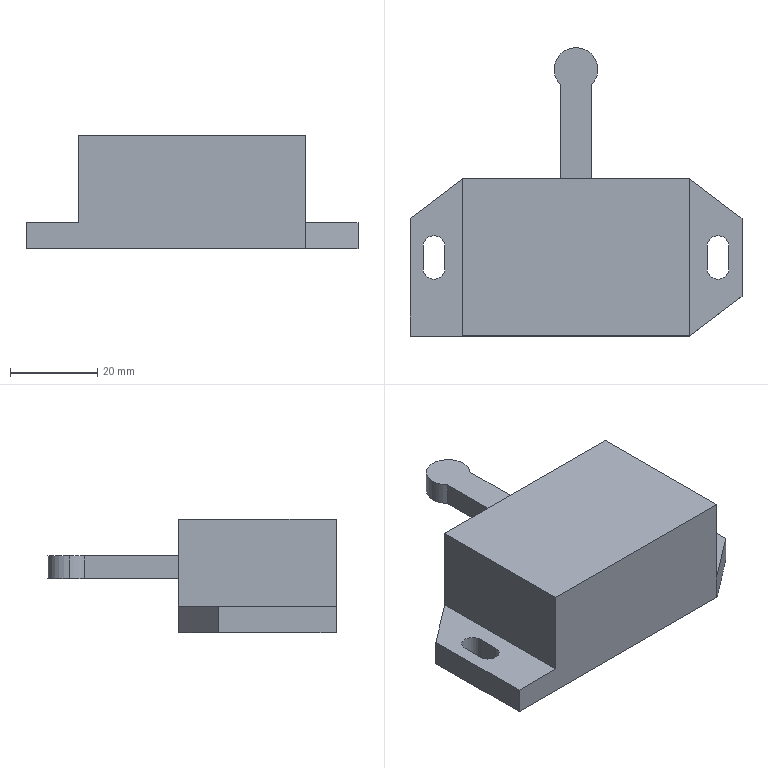Part | SolidWorks | features BaseBody 1 | 1 solid | 28 faces | box 76 x 66 x 26 mm | volume 53615 mm3 | plane 21 | cylinder 7 | commonest cylinder face diameters 5 x4 10 x3
STEP:
#1=CARTESIAN_POINT('',(-5.,43.,12.393));
#2=VERTEX_POINT('',#1);
#3=CARTESIAN_POINT('',(-5.,43.,17.607));
#4=VERTEX_POINT('',#3);
#5=CARTESIAN_POINT('',(-5.,43.,-1.75));
#6=DIRECTION('',(0.,0.,1.));
#7=VECTOR('',#6,1000.);
#8=LINE('',#5,#7);
#9=EDGE_CURVE('',#2,#4,#8,.T.);
#10=ORIENTED_EDGE('',*,*,#9,.F.);
#11=CARTESIAN_POINT('',(-3.61,39.541,12.393));
#12=VERTEX_POINT('',#11);
#13=CARTESIAN_POINT('',(0.,43.,12.393));
#14=DIRECTION('',(0.,0.,-1.));
#15=DIRECTION('',(1.,0.,0.));
#16=AXIS2_PLACEMENT_3D('',#13,#14,#15);
#17=CIRCLE('',#16,5.);
#18=EDGE_CURVE('',#12,#2,#17,.T.);
#19=ORIENTED_EDGE('',*,*,#18,.F.);
#20=CARTESIAN_POINT('',(-3.61,39.541,17.607));
#21=VERTEX_POINT('',#20);
#22=CARTESIAN_POINT('',(-3.61,39.541,-1.75));
#23=DIRECTION('',(0.,0.,-1.));
#24=VECTOR('',#23,1000.);
#25=LINE('',#22,#24);
#26=EDGE_CURVE('',#21,#12,#25,.T.);
#27=ORIENTED_EDGE('',*,*,#26,.F.);
#28=CARTESIAN_POINT('',(0.,43.,17.607));
#29=DIRECTION('',(0.,0.,1.));
#30=DIRECTION('',(1.,0.,0.));
#31=AXIS2_PLACEMENT_3D('',#28,#29,#30);
#32=CIRCLE('',#31,5.);
#33=EDGE_CURVE('',#4,#21,#32,.T.);
#34=ORIENTED_EDGE('',*,*,#33,.F.);
#35=EDGE_LOOP('',(#10,#19,#27,#34));
#36=FACE_OUTER_BOUND('',#35,.T.);
#37=CARTESIAN_POINT('',(0.,43.,-1.75));
#38=DIRECTION('',(0.,0.,1.));
#39=DIRECTION('',(1.,0.,0.));
#40=AXIS2_PLACEMENT_3D('',#37,#38,#39);
#41=CYLINDRICAL_SURFACE('',#40,5.);
#42=ADVANCED_FACE('',(#36),#41,.T.);
#43=CARTESIAN_POINT('',(3.61,39.541,17.607));
#44=VERTEX_POINT('',#43);
#45=CARTESIAN_POINT('',(3.61,18.,17.607));
#46=VERTEX_POINT('',#45);
#47=CARTESIAN_POINT('',(3.61,43.,17.607));
#48=DIRECTION('',(0.,-1.,0.));
#49=VECTOR('',#48,1000.);
#50=LINE('',#47,#49);
#51=EDGE_CURVE('',#44,#46,#50,.T.);
#52=ORIENTED_EDGE('',*,*,#51,.F.);
#53=CARTESIAN_POINT('',(5.,43.,17.607));
#54=VERTEX_POINT('',#53);
#55=CARTESIAN_POINT('',(0.,43.,17.607));
#56=DIRECTION('',(0.,0.,1.));
#57=DIRECTION('',(1.,0.,0.));
#58=AXIS2_PLACEMENT_3D('',#55,#56,#57);
#59=CIRCLE('',#58,5.);
#60=EDGE_CURVE('',#44,#54,#59,.T.);
#61=ORIENTED_EDGE('',*,*,#60,.T.);
#62=CARTESIAN_POINT('',(0.,43.,17.607));
#63=DIRECTION('',(0.,0.,1.));
#64=DIRECTION('',(1.,0.,0.));
#65=AXIS2_PLACEMENT_3D('',#62,#63,#64);
#66=CIRCLE('',#65,5.);
#67=EDGE_CURVE('',#54,#4,#66,.T.);
#68=ORIENTED_EDGE('',*,*,#67,.T.);
#69=ORIENTED_EDGE('',*,*,#33,.T.);
#70=CARTESIAN_POINT('',(-3.61,18.,17.607));
#71=VERTEX_POINT('',#70);
#72=CARTESIAN_POINT('',(-3.61,43.,17.607));
#73=DIRECTION('',(0.,-1.,0.));
#74=VECTOR('',#73,1000.);
#75=LINE('',#72,#74);
#76=EDGE_CURVE('',#21,#71,#75,.T.);
#77=ORIENTED_EDGE('',*,*,#76,.T.);
#78=CARTESIAN_POINT('',(-3.61,18.,17.607));
#79=DIRECTION('',(1.,0.,0.));
#80=VECTOR('',#79,1000.);
#81=LINE('',#78,#80);
#82=EDGE_CURVE('',#71,#46,#81,.T.);
#83=ORIENTED_EDGE('',*,*,#82,.T.);
#84=EDGE_LOOP('',(#52,#61,#68,#69,#77,#83));
#85=FACE_OUTER_BOUND('',#84,.T.);
#86=CARTESIAN_POINT('',(-3.61,43.,17.607));
#87=DIRECTION('',(0.,0.,-1.));
#88=DIRECTION('',(-1.,0.,0.));
#89=AXIS2_PLACEMENT_3D('',#86,#87,#88);
#90=PLANE('',#89);
#91=ADVANCED_FACE('',(#85),#90,.F.);
#92=ORIENTED_EDGE('',*,*,#76,.F.);
#93=ORIENTED_EDGE('',*,*,#26,.T.);
#94=CARTESIAN_POINT('',(-3.61,18.,12.393));
#95=VERTEX_POINT('',#94);
#96=CARTESIAN_POINT('',(-3.61,43.,12.393));
#97=DIRECTION('',(0.,-1.,0.));
#98=VECTOR('',#97,1000.);
#99=LINE('',#96,#98);
#100=EDGE_CURVE('',#12,#95,#99,.T.);
#101=ORIENTED_EDGE('',*,*,#100,.T.);
#102=CARTESIAN_POINT('',(-3.61,18.,12.393));
#103=DIRECTION('',(0.,0.,1.));
#104=VECTOR('',#103,1000.);
#105=LINE('',#102,#104);
#106=EDGE_CURVE('',#95,#71,#105,.T.);
#107=ORIENTED_EDGE('',*,*,#106,.T.);
#108=EDGE_LOOP('',(#92,#93,#101,#107));
#109=FACE_OUTER_BOUND('',#108,.T.);
#110=CARTESIAN_POINT('',(-3.61,43.,12.393));
#111=DIRECTION('',(1.,0.,0.));
#112=DIRECTION('',(0.,1.,0.));
#113=AXIS2_PLACEMENT_3D('',#110,#111,#112);
#114=PLANE('',#113);
#115=ADVANCED_FACE('',(#109),#114,.F.);
#116=ORIENTED_EDGE('',*,*,#18,.T.);
#117=CARTESIAN_POINT('',(5.,43.,12.393));
#118=VERTEX_POINT('',#117);
#119=CARTESIAN_POINT('',(0.,43.,12.393));
#120=DIRECTION('',(0.,0.,-1.));
#121=DIRECTION('',(1.,0.,0.));
#122=AXIS2_PLACEMENT_3D('',#119,#120,#121);
#123=CIRCLE('',#122,5.);
#124=EDGE_CURVE('',#2,#118,#123,.T.);
#125=ORIENTED_EDGE('',*,*,#124,.T.);
#126=CARTESIAN_POINT('',(3.61,39.541,12.393));
#127=VERTEX_POINT('',#126);
#128=CARTESIAN_POINT('',(0.,43.,12.393));
#129=DIRECTION('',(0.,0.,-1.));
#130=DIRECTION('',(1.,0.,0.));
#131=AXIS2_PLACEMENT_3D('',#128,#129,#130);
#132=CIRCLE('',#131,5.);
#133=EDGE_CURVE('',#118,#127,#132,.T.);
#134=ORIENTED_EDGE('',*,*,#133,.T.);
#135=CARTESIAN_POINT('',(3.61,18.,12.393));
#136=VERTEX_POINT('',#135);
#137=CARTESIAN_POINT('',(3.61,43.,12.393));
#138=DIRECTION('',(0.,-1.,0.));
#139=VECTOR('',#138,1000.);
#140=LINE('',#137,#139);
#141=EDGE_CURVE('',#127,#136,#140,.T.);
#142=ORIENTED_EDGE('',*,*,#141,.T.);
#143=CARTESIAN_POINT('',(-3.61,18.,12.393));
#144=DIRECTION('',(-1.,0.,0.));
#145=VECTOR('',#144,1000.);
#146=LINE('',#143,#145);
#147=EDGE_CURVE('',#136,#95,#146,.T.);
#148=ORIENTED_EDGE('',*,*,#147,.T.);
#149=ORIENTED_EDGE('',*,*,#100,.F.);
#150=EDGE_LOOP('',(#116,#125,#134,#142,#148,#149));
#151=FACE_OUTER_BOUND('',#150,.T.);
#152=CARTESIAN_POINT('',(-3.61,43.,12.393));
#153=DIRECTION('',(0.,0.,1.));
#154=DIRECTION('',(1.,0.,0.));
#155=AXIS2_PLACEMENT_3D('',#152,#153,#154);
#156=PLANE('',#155);
#157=ADVANCED_FACE('',(#151),#156,.F.);
#158=ORIENTED_EDGE('',*,*,#141,.F.);
#159=CARTESIAN_POINT('',(3.61,39.541,-1.75));
#160=DIRECTION('',(0.,0.,1.));
#161=VECTOR('',#160,1000.);
#162=LINE('',#159,#161);
#163=EDGE_CURVE('',#127,#44,#162,.T.);
#164=ORIENTED_EDGE('',*,*,#163,.T.);
#165=ORIENTED_EDGE('',*,*,#51,.T.);
#166=CARTESIAN_POINT('',(3.61,18.,12.393));
#167=DIRECTION('',(0.,0.,-1.));
#168=VECTOR('',#167,1000.);
#169=LINE('',#166,#168);
#170=EDGE_CURVE('',#46,#136,#169,.T.);
#171=ORIENTED_EDGE('',*,*,#170,.T.);
#172=EDGE_LOOP('',(#158,#164,#165,#171));
#173=FACE_OUTER_BOUND('',#172,.T.);
#174=CARTESIAN_POINT('',(3.61,43.,12.393));
#175=DIRECTION('',(-1.,0.,0.));
#176=DIRECTION('',(0.,1.,0.));
#177=AXIS2_PLACEMENT_3D('',#174,#175,#176);
#178=PLANE('',#177);
#179=ADVANCED_FACE('',(#173),#178,.F.);
#180=CARTESIAN_POINT('',(26.062,-18.,26.));
#181=VERTEX_POINT('',#180);
#182=CARTESIAN_POINT('',(26.062,18.,26.));
#183=VERTEX_POINT('',#182);
#184=CARTESIAN_POINT('',(26.062,-18.,26.));
#185=DIRECTION('',(0.,1.,0.));
#186=VECTOR('',#185,1000.);
#187=LINE('',#184,#186);
#188=EDGE_CURVE('',#181,#183,#187,.T.);
#189=ORIENTED_EDGE('',*,*,#188,.T.);
#190=CARTESIAN_POINT('',(-26.062,18.,26.));
#191=VERTEX_POINT('',#190);
#192=CARTESIAN_POINT('',(-26.062,18.,26.));
#193=DIRECTION('',(-1.,0.,0.));
#194=VECTOR('',#193,1000.);
#195=LINE('',#192,#194);
#196=EDGE_CURVE('',#183,#191,#195,.T.);
#197=ORIENTED_EDGE('',*,*,#196,.T.);
#198=CARTESIAN_POINT('',(-26.062,-18.,26.));
#199=VERTEX_POINT('',#198);
#200=CARTESIAN_POINT('',(-26.062,-18.,26.));
#201=DIRECTION('',(0.,-1.,0.));
#202=VECTOR('',#201,1000.);
#203=LINE('',#200,#202);
#204=EDGE_CURVE('',#191,#199,#203,.T.);
#205=ORIENTED_EDGE('',*,*,#204,.T.);
#206=CARTESIAN_POINT('',(-26.062,-18.,26.));
#207=DIRECTION('',(1.,0.,0.));
#208=VECTOR('',#207,1000.);
#209=LINE('',#206,#208);
#210=EDGE_CURVE('',#199,#181,#209,.T.);
#211=ORIENTED_EDGE('',*,*,#210,.T.);
#212=EDGE_LOOP('',(#189,#197,#205,#211));
#213=FACE_OUTER_BOUND('',#212,.T.);
#214=CARTESIAN_POINT('',(0.,0.,26.));
#215=DIRECTION('',(0.,0.,-1.));
#216=DIRECTION('',(0.,-1.,0.));
#217=AXIS2_PLACEMENT_3D('',#214,#215,#216);
#218=PLANE('',#217);
#219=ADVANCED_FACE('',(#213),#218,.F.);
#220=CARTESIAN_POINT('',(-26.062,18.,6.));
#221=VERTEX_POINT('',#220);
#222=CARTESIAN_POINT('',(-26.062,-18.,6.));
#223=VERTEX_POINT('',#222);
#224=CARTESIAN_POINT('',(-26.062,-18.,6.));
#225=DIRECTION('',(0.,-1.,0.));
#226=VECTOR('',#225,1000.);
#227=LINE('',#224,#226);
#228=EDGE_CURVE('',#221,#223,#227,.T.);
#229=ORIENTED_EDGE('',*,*,#228,.T.);
#230=CARTESIAN_POINT('',(-26.062,-18.,26.));
#231=DIRECTION('',(0.,0.,-1.));
#232=VECTOR('',#231,1000.);
#233=LINE('',#230,#232);
#234=EDGE_CURVE('',#199,#223,#233,.T.);
#235=ORIENTED_EDGE('',*,*,#234,.F.);
#236=ORIENTED_EDGE('',*,*,#204,.F.);
#237=CARTESIAN_POINT('',(-26.062,18.,26.));
#238=DIRECTION('',(0.,0.,-1.));
#239=VECTOR('',#238,1000.);
#240=LINE('',#237,#239);
#241=EDGE_CURVE('',#191,#221,#240,.T.);
#242=ORIENTED_EDGE('',*,*,#241,.T.);
#243=EDGE_LOOP('',(#229,#235,#236,#242));
#244=FACE_OUTER_BOUND('',#243,.T.);
#245=CARTESIAN_POINT('',(-26.062,-18.,26.));
#246=DIRECTION('',(1.,0.,0.));
#247=DIRECTION('',(0.,1.,0.));
#248=AXIS2_PLACEMENT_3D('',#245,#246,#247);
#249=PLANE('',#248);
#250=ADVANCED_FACE('',(#244),#249,.F.);
#251=CARTESIAN_POINT('',(26.062,-18.,6.));
#252=VERTEX_POINT('',#251);
#253=CARTESIAN_POINT('',(26.062,18.,6.));
#254=VERTEX_POINT('',#253);
#255=CARTESIAN_POINT('',(26.062,-18.,6.));
#256=DIRECTION('',(0.,1.,0.));
#257=VECTOR('',#256,1000.);
#258=LINE('',#255,#257);
#259=EDGE_CURVE('',#252,#254,#258,.T.);
#260=ORIENTED_EDGE('',*,*,#259,.T.);
#261=CARTESIAN_POINT('',(26.062,18.,26.));
#262=DIRECTION('',(0.,0.,-1.));
#263=VECTOR('',#262,1000.);
#264=LINE('',#261,#263);
#265=EDGE_CURVE('',#183,#254,#264,.T.);
#266=ORIENTED_EDGE('',*,*,#265,.F.);
#267=ORIENTED_EDGE('',*,*,#188,.F.);
#268=CARTESIAN_POINT('',(26.062,-18.,26.));
#269=DIRECTION('',(0.,0.,-1.));
#270=VECTOR('',#269,1000.);
#271=LINE('',#268,#270);
#272=EDGE_CURVE('',#181,#252,#271,.T.);
#273=ORIENTED_EDGE('',*,*,#272,.T.);
#274=EDGE_LOOP('',(#260,#266,#267,#273));
#275=FACE_OUTER_BOUND('',#274,.T.);
#276=CARTESIAN_POINT('',(26.062,-18.,26.));
#277=DIRECTION('',(-1.,0.,0.));
#278=DIRECTION('',(0.,0.,1.));
#279=AXIS2_PLACEMENT_3D('',#276,#277,#278);
#280=PLANE('',#279);
#281=ADVANCED_FACE('',(#275),#280,.F.);
#282=CARTESIAN_POINT('',(35.,-2.5,0.));
#283=VERTEX_POINT('',#282);
#284=CARTESIAN_POINT('',(35.,2.5,0.));
#285=VERTEX_POINT('',#284);
#286=CARTESIAN_POINT('',(35.,2.5,0.));
#287=DIRECTION('',(0.,1.,0.));
#288=VECTOR('',#287,1000.);
#289=LINE('',#286,#288);
#290=EDGE_CURVE('',#283,#285,#289,.T.);
#291=ORIENTED_EDGE('',*,*,#290,.F.);
#292=CARTESIAN_POINT('',(35.,-2.5,6.));
#293=VERTEX_POINT('',#292);
#294=CARTESIAN_POINT('',(35.,-2.5,6.));
#295=DIRECTION('',(0.,0.,-1.));
#296=VECTOR('',#295,1000.);
#297=LINE('',#294,#296);
#298=EDGE_CURVE('',#293,#283,#297,.T.);
#299=ORIENTED_EDGE('',*,*,#298,.F.);
#300=CARTESIAN_POINT('',(35.,2.5,6.));
#301=VERTEX_POINT('',#300);
#302=CARTESIAN_POINT('',(35.,2.5,6.));
#303=DIRECTION('',(0.,1.,0.));
#304=VECTOR('',#303,1000.);
#305=LINE('',#302,#304);
#306=EDGE_CURVE('',#293,#301,#305,.T.);
#307=ORIENTED_EDGE('',*,*,#306,.T.);
#308=CARTESIAN_POINT('',(35.,2.5,6.));
#309=DIRECTION('',(0.,0.,-1.));
#310=VECTOR('',#309,1000.);
#311=LINE('',#308,#310);
#312=EDGE_CURVE('',#301,#285,#311,.T.);
#313=ORIENTED_EDGE('',*,*,#312,.T.);
#314=EDGE_LOOP('',(#291,#299,#307,#313));
#315=FACE_OUTER_BOUND('',#314,.T.);
#316=CARTESIAN_POINT('',(35.,2.5,6.));
#317=DIRECTION('',(-1.,0.,0.));
#318=DIRECTION('',(0.,0.,1.));
#319=AXIS2_PLACEMENT_3D('',#316,#317,#318);
#320=PLANE('',#319);
#321=ADVANCED_FACE('',(#315),#320,.T.);
#322=CARTESIAN_POINT('',(30.,-2.5,0.));
#323=VERTEX_POINT('',#322);
#324=CARTESIAN_POINT('',(32.5,-2.5,0.));
#325=DIRECTION('',(0.,0.,1.));
#326=DIRECTION('',(-1.,0.,0.));
#327=AXIS2_PLACEMENT_3D('',#324,#325,#326);
#328=CIRCLE('',#327,2.5);
#329=EDGE_CURVE('',#323,#283,#328,.T.);
#330=ORIENTED_EDGE('',*,*,#329,.F.);
#331=CARTESIAN_POINT('',(30.,-2.5,6.));
#332=VERTEX_POINT('',#331);
#333=CARTESIAN_POINT('',(30.,-2.5,6.));
#334=DIRECTION('',(0.,0.,-1.));
#335=VECTOR('',#334,1000.);
#336=LINE('',#333,#335);
#337=EDGE_CURVE('',#332,#323,#336,.T.);
#338=ORIENTED_EDGE('',*,*,#337,.F.);
#339=CARTESIAN_POINT('',(32.5,-2.5,6.));
#340=DIRECTION('',(0.,0.,1.));
#341=DIRECTION('',(-1.,0.,0.));
#342=AXIS2_PLACEMENT_3D('',#339,#340,#341);
#343=CIRCLE('',#342,2.5);
#344=EDGE_CURVE('',#332,#293,#343,.T.);
#345=ORIENTED_EDGE('',*,*,#344,.T.);
#346=ORIENTED_EDGE('',*,*,#298,.T.);
#347=EDGE_LOOP('',(#330,#338,#345,#346));
#348=FACE_OUTER_BOUND('',#347,.T.);
#349=CARTESIAN_POINT('',(32.5,-2.5,6.));
#350=DIRECTION('',(0.,0.,-1.));
#351=DIRECTION('',(-1.,0.,0.));
#352=AXIS2_PLACEMENT_3D('',#349,#350,#351);
#353=CYLINDRICAL_SURFACE('',#352,2.5);
#354=ADVANCED_FACE('',(#348),#353,.F.);
#355=CARTESIAN_POINT('',(30.,2.5,0.));
#356=VERTEX_POINT('',#355);
#357=CARTESIAN_POINT('',(30.,2.5,0.));
#358=DIRECTION('',(0.,-1.,0.));
#359=VECTOR('',#358,1000.);
#360=LINE('',#357,#359);
#361=EDGE_CURVE('',#356,#323,#360,.T.);
#362=ORIENTED_EDGE('',*,*,#361,.F.);
#363=CARTESIAN_POINT('',(30.,2.5,6.));
#364=VERTEX_POINT('',#363);
#365=CARTESIAN_POINT('',(30.,2.5,6.));
#366=DIRECTION('',(0.,0.,-1.));
#367=VECTOR('',#366,1000.);
#368=LINE('',#365,#367);
#369=EDGE_CURVE('',#364,#356,#368,.T.);
#370=ORIENTED_EDGE('',*,*,#369,.F.);
#371=CARTESIAN_POINT('',(30.,2.5,6.));
#372=DIRECTION('',(0.,-1.,0.));
#373=VECTOR('',#372,1000.);
#374=LINE('',#371,#373);
#375=EDGE_CURVE('',#364,#332,#374,.T.);
#376=ORIENTED_EDGE('',*,*,#375,.T.);
#377=ORIENTED_EDGE('',*,*,#337,.T.);
#378=EDGE_LOOP('',(#362,#370,#376,#377));
#379=FACE_OUTER_BOUND('',#378,.T.);
#380=CARTESIAN_POINT('',(30.,2.5,6.));
#381=DIRECTION('',(1.,0.,0.));
#382=DIRECTION('',(0.,1.,0.));
#383=AXIS2_PLACEMENT_3D('',#380,#381,#382);
#384=PLANE('',#383);
#385=ADVANCED_FACE('',(#379),#384,.T.);
#386=CARTESIAN_POINT('',(32.5,2.5,0.));
#387=DIRECTION('',(0.,0.,1.));
#388=DIRECTION('',(-1.,0.,0.));
#389=AXIS2_PLACEMENT_3D('',#386,#387,#388);
#390=CIRCLE('',#389,2.5);
#391=EDGE_CURVE('',#285,#356,#390,.T.);
#392=ORIENTED_EDGE('',*,*,#391,.F.);
#393=ORIENTED_EDGE('',*,*,#312,.F.);
#394=CARTESIAN_POINT('',(32.5,2.5,6.));
#395=DIRECTION('',(0.,0.,1.));
#396=DIRECTION('',(-1.,0.,0.));
#397=AXIS2_PLACEMENT_3D('',#394,#395,#396);
#398=CIRCLE('',#397,2.5);
#399=EDGE_CURVE('',#301,#364,#398,.T.);
#400=ORIENTED_EDGE('',*,*,#399,.T.);
#401=ORIENTED_EDGE('',*,*,#369,.T.);
#402=EDGE_LOOP('',(#392,#393,#400,#401));
#403=FACE_OUTER_BOUND('',#402,.T.);
#404=CARTESIAN_POINT('',(32.5,2.5,6.));
#405=DIRECTION('',(0.,0.,-1.));
#406=DIRECTION('',(-1.,0.,0.));
#407=AXIS2_PLACEMENT_3D('',#404,#405,#406);
#408=CYLINDRICAL_SURFACE('',#407,2.5);
#409=ADVANCED_FACE('',(#403),#408,.F.);
#410=CARTESIAN_POINT('',(-30.,-2.5,0.));
#411=VERTEX_POINT('',#410);
#412=CARTESIAN_POINT('',(-30.,2.5,0.));
#413=VERTEX_POINT('',#412);
#414=CARTESIAN_POINT('',(-30.,2.5,0.));
#415=DIRECTION('',(0.,1.,0.));
#416=VECTOR('',#415,1000.);
#417=LINE('',#414,#416);
#418=EDGE_CURVE('',#411,#413,#417,.T.);
#419=ORIENTED_EDGE('',*,*,#418,.F.);
#420=CARTESIAN_POINT('',(-30.,-2.5,6.));
#421=VERTEX_POINT('',#420);
#422=CARTESIAN_POINT('',(-30.,-2.5,6.));
#423=DIRECTION('',(0.,0.,-1.));
#424=VECTOR('',#423,1000.);
#425=LINE('',#422,#424);
#426=EDGE_CURVE('',#421,#411,#425,.T.);
#427=ORIENTED_EDGE('',*,*,#426,.F.);
#428=CARTESIAN_POINT('',(-30.,2.5,6.));
#429=VERTEX_POINT('',#428);
#430=CARTESIAN_POINT('',(-30.,2.5,6.));
#431=DIRECTION('',(0.,1.,0.));
#432=VECTOR('',#431,1000.);
#433=LINE('',#430,#432);
#434=EDGE_CURVE('',#421,#429,#433,.T.);
#435=ORIENTED_EDGE('',*,*,#434,.T.);
#436=CARTESIAN_POINT('',(-30.,2.5,6.));
#437=DIRECTION('',(0.,0.,-1.));
#438=VECTOR('',#437,1000.);
#439=LINE('',#436,#438);
#440=EDGE_CURVE('',#429,#413,#439,.T.);
#441=ORIENTED_EDGE('',*,*,#440,.T.);
#442=EDGE_LOOP('',(#419,#427,#435,#441));
#443=FACE_OUTER_BOUND('',#442,.T.);
#444=CARTESIAN_POINT('',(-30.,2.5,6.));
#445=DIRECTION('',(-1.,0.,0.));
#446=DIRECTION('',(0.,0.,1.));
#447=AXIS2_PLACEMENT_3D('',#444,#445,#446);
#448=PLANE('',#447);
#449=ADVANCED_FACE('',(#443),#448,.T.);
#450=CARTESIAN_POINT('',(-35.,-2.5,0.));
#451=VERTEX_POINT('',#450);
#452=CARTESIAN_POINT('',(-32.5,-2.5,0.));
#453=DIRECTION('',(0.,0.,1.));
#454=DIRECTION('',(1.,0.,0.));
#455=AXIS2_PLACEMENT_3D('',#452,#453,#454);
#456=CIRCLE('',#455,2.5);
#457=EDGE_CURVE('',#451,#411,#456,.T.);
#458=ORIENTED_EDGE('',*,*,#457,.F.);
#459=CARTESIAN_POINT('',(-35.,-2.5,6.));
#460=VERTEX_POINT('',#459);
#461=CARTESIAN_POINT('',(-35.,-2.5,6.));
#462=DIRECTION('',(0.,0.,-1.));
#463=VECTOR('',#462,1000.);
#464=LINE('',#461,#463);
#465=EDGE_CURVE('',#460,#451,#464,.T.);
#466=ORIENTED_EDGE('',*,*,#465,.F.);
#467=CARTESIAN_POINT('',(-32.5,-2.5,6.));
#468=DIRECTION('',(0.,0.,1.));
#469=DIRECTION('',(1.,0.,0.));
#470=AXIS2_PLACEMENT_3D('',#467,#468,#469);
#471=CIRCLE('',#470,2.5);
#472=EDGE_CURVE('',#460,#421,#471,.T.);
#473=ORIENTED_EDGE('',*,*,#472,.T.);
#474=ORIENTED_EDGE('',*,*,#426,.T.);
#475=EDGE_LOOP('',(#458,#466,#473,#474));
#476=FACE_OUTER_BOUND('',#475,.T.);
#477=CARTESIAN_POINT('',(-32.5,-2.5,6.));
#478=DIRECTION('',(0.,0.,-1.));
#479=DIRECTION('',(-1.,0.,0.));
#480=AXIS2_PLACEMENT_3D('',#477,#478,#479);
#481=CYLINDRICAL_SURFACE('',#480,2.5);
#482=ADVANCED_FACE('',(#476),#481,.F.);
#483=CARTESIAN_POINT('',(-35.,2.5,0.));
#484=VERTEX_POINT('',#483);
#485=CARTESIAN_POINT('',(-35.,2.5,0.));
#486=DIRECTION('',(0.,-1.,0.));
#487=VECTOR('',#486,1000.);
#488=LINE('',#485,#487);
#489=EDGE_CURVE('',#484,#451,#488,.T.);
#490=ORIENTED_EDGE('',*,*,#489,.F.);
#491=CARTESIAN_POINT('',(-35.,2.5,6.));
#492=VERTEX_POINT('',#491);
#493=CARTESIAN_POINT('',(-35.,2.5,6.));
#494=DIRECTION('',(0.,0.,-1.));
#495=VECTOR('',#494,1000.);
#496=LINE('',#493,#495);
#497=EDGE_CURVE('',#492,#484,#496,.T.);
#498=ORIENTED_EDGE('',*,*,#497,.F.);
#499=CARTESIAN_POINT('',(-35.,2.5,6.));
#500=DIRECTION('',(0.,-1.,0.));
#501=VECTOR('',#500,1000.);
#502=LINE('',#499,#501);
#503=EDGE_CURVE('',#492,#460,#502,.T.);
#504=ORIENTED_EDGE('',*,*,#503,.T.);
#505=ORIENTED_EDGE('',*,*,#465,.T.);
#506=EDGE_LOOP('',(#490,#498,#504,#505));
#507=FACE_OUTER_BOUND('',#506,.T.);
#508=CARTESIAN_POINT('',(-35.,2.5,6.));
#509=DIRECTION('',(1.,0.,0.));
#510=DIRECTION('',(0.,1.,0.));
#511=AXIS2_PLACEMENT_3D('',#508,#509,#510);
#512=PLANE('',#511);
#513=ADVANCED_FACE('',(#507),#512,.T.);
#514=CARTESIAN_POINT('',(-32.5,2.5,0.));
#515=DIRECTION('',(0.,0.,1.));
#516=DIRECTION('',(1.,0.,0.));
#517=AXIS2_PLACEMENT_3D('',#514,#515,#516);
#518=CIRCLE('',#517,2.5);
#519=EDGE_CURVE('',#413,#484,#518,.T.);
#520=ORIENTED_EDGE('',*,*,#519,.F.);
#521=ORIENTED_EDGE('',*,*,#440,.F.);
#522=CARTESIAN_POINT('',(-32.5,2.5,6.));
#523=DIRECTION('',(0.,0.,1.));
#524=DIRECTION('',(1.,0.,0.));
#525=AXIS2_PLACEMENT_3D('',#522,#523,#524);
#526=CIRCLE('',#525,2.5);
#527=EDGE_CURVE('',#429,#492,#526,.T.);
#528=ORIENTED_EDGE('',*,*,#527,.T.);
#529=ORIENTED_EDGE('',*,*,#497,.T.);
#530=EDGE_LOOP('',(#520,#521,#528,#529));
#531=FACE_OUTER_BOUND('',#530,.T.);
#532=CARTESIAN_POINT('',(-32.5,2.5,6.));
#533=DIRECTION('',(0.,0.,-1.));
#534=DIRECTION('',(-1.,0.,0.));
#535=AXIS2_PLACEMENT_3D('',#532,#533,#534);
#536=CYLINDRICAL_SURFACE('',#535,2.5);
#537=ADVANCED_FACE('',(#531),#536,.F.);
#538=CARTESIAN_POINT('',(-38.,8.923,0.));
#539=VERTEX_POINT('',#538);
#540=CARTESIAN_POINT('',(-38.,-18.,0.));
#541=VERTEX_POINT('',#540);
#542=CARTESIAN_POINT('',(-38.,8.923,0.));
#543=DIRECTION('',(0.,-1.,0.));
#544=VECTOR('',#543,1000.);
#545=LINE('',#542,#544);
#546=EDGE_CURVE('',#539,#541,#545,.T.);
#547=ORIENTED_EDGE('',*,*,#546,.T.);
#548=CARTESIAN_POINT('',(-38.,-18.,6.));
#549=VERTEX_POINT('',#548);
#550=CARTESIAN_POINT('',(-38.,-18.,6.));
#551=DIRECTION('',(0.,0.,-1.));
#552=VECTOR('',#551,1000.);
#553=LINE('',#550,#552);
#554=EDGE_CURVE('',#549,#541,#553,.T.);
#555=ORIENTED_EDGE('',*,*,#554,.F.);
#556=CARTESIAN_POINT('',(-38.,8.923,6.));
#557=VERTEX_POINT('',#556);
#558=CARTESIAN_POINT('',(-38.,8.923,6.));
#559=DIRECTION('',(0.,-1.,0.));
#560=VECTOR('',#559,1000.);
#561=LINE('',#558,#560);
#562=EDGE_CURVE('',#557,#549,#561,.T.);
#563=ORIENTED_EDGE('',*,*,#562,.F.);
#564=CARTESIAN_POINT('',(-38.,8.923,6.));
#565=DIRECTION('',(0.,0.,-1.));
#566=VECTOR('',#565,1000.);
#567=LINE('',#564,#566);
#568=EDGE_CURVE('',#557,#539,#567,.T.);
#569=ORIENTED_EDGE('',*,*,#568,.T.);
#570=EDGE_LOOP('',(#547,#555,#563,#569));
#571=FACE_OUTER_BOUND('',#570,.T.);
#572=CARTESIAN_POINT('',(-38.,8.923,6.));
#573=DIRECTION('',(1.,0.,0.));
#574=DIRECTION('',(0.,-1.,0.));
#575=AXIS2_PLACEMENT_3D('',#572,#573,#574);
#576=PLANE('',#575);
#577=ADVANCED_FACE('',(#571),#576,.F.);
#578=CARTESIAN_POINT('',(-26.062,18.,0.));
#579=VERTEX_POINT('',#578);
#580=CARTESIAN_POINT('',(-26.062,18.,0.));
#581=DIRECTION('',(-0.796,-0.6053,0.));
#582=VECTOR('',#581,1000.);
#583=LINE('',#580,#582);
#584=EDGE_CURVE('',#579,#539,#583,.T.);
#585=ORIENTED_EDGE('',*,*,#584,.T.);
#586=ORIENTED_EDGE('',*,*,#568,.F.);
#587=CARTESIAN_POINT('',(-26.062,18.,6.));
#588=DIRECTION('',(-0.796,-0.6053,0.));
#589=VECTOR('',#588,1000.);
#590=LINE('',#587,#589);
#591=EDGE_CURVE('',#221,#557,#590,.T.);
#592=ORIENTED_EDGE('',*,*,#591,.F.);
#593=CARTESIAN_POINT('',(-26.062,18.,6.));
#594=DIRECTION('',(0.,0.,-1.));
#595=VECTOR('',#594,1000.);
#596=LINE('',#593,#595);
#597=EDGE_CURVE('',#221,#579,#596,.T.);
#598=ORIENTED_EDGE('',*,*,#597,.T.);
#599=EDGE_LOOP('',(#585,#586,#592,#598));
#600=FACE_OUTER_BOUND('',#599,.T.);
#601=CARTESIAN_POINT('',(-26.062,18.,6.));
#602=DIRECTION('',(0.6053,-0.796,0.));
#603=DIRECTION('',(0.,0.,-1.));
#604=AXIS2_PLACEMENT_3D('',#601,#602,#603);
#605=PLANE('',#604);
#606=ADVANCED_FACE('',(#600),#605,.F.);
#607=CARTESIAN_POINT('',(38.,8.923,0.));
#608=VERTEX_POINT('',#607);
#609=CARTESIAN_POINT('',(26.062,18.,0.));
#610=VERTEX_POINT('',#609);
#611=CARTESIAN_POINT('',(26.062,18.,0.));
#612=DIRECTION('',(-0.796,0.6053,0.));
#613=VECTOR('',#612,1000.);
#614=LINE('',#611,#613);
#615=EDGE_CURVE('',#608,#610,#614,.T.);
#616=ORIENTED_EDGE('',*,*,#615,.T.);
#617=CARTESIAN_POINT('',(26.062,18.,6.));
#618=DIRECTION('',(0.,0.,-1.));
#619=VECTOR('',#618,1000.);
#620=LINE('',#617,#619);
#621=EDGE_CURVE('',#254,#610,#620,.T.);
#622=ORIENTED_EDGE('',*,*,#621,.F.);
#623=CARTESIAN_POINT('',(38.,8.923,6.));
#624=VERTEX_POINT('',#623);
#625=CARTESIAN_POINT('',(26.062,18.,6.));
#626=DIRECTION('',(-0.796,0.6053,0.));
#627=VECTOR('',#626,1000.);
#628=LINE('',#625,#627);
#629=EDGE_CURVE('',#624,#254,#628,.T.);
#630=ORIENTED_EDGE('',*,*,#629,.F.);
#631=CARTESIAN_POINT('',(38.,8.923,6.));
#632=DIRECTION('',(0.,0.,-1.));
#633=VECTOR('',#632,1000.);
#634=LINE('',#631,#633);
#635=EDGE_CURVE('',#624,#608,#634,.T.);
#636=ORIENTED_EDGE('',*,*,#635,.T.);
#637=EDGE_LOOP('',(#616,#622,#630,#636));
#638=FACE_OUTER_BOUND('',#637,.T.);
#639=CARTESIAN_POINT('',(26.062,18.,6.));
#640=DIRECTION('',(-0.6053,-0.796,0.));
#641=DIRECTION('',(-0.796,0.6053,0.));
#642=AXIS2_PLACEMENT_3D('',#639,#640,#641);
#643=PLANE('',#642);
#644=ADVANCED_FACE('',(#638),#643,.F.);
#645=CARTESIAN_POINT('',(38.,-8.923,0.));
#646=VERTEX_POINT('',#645);
#647=CARTESIAN_POINT('',(38.,8.923,0.));
#648=DIRECTION('',(0.,1.,0.));
#649=VECTOR('',#648,1000.);
#650=LINE('',#647,#649);
#651=EDGE_CURVE('',#646,#608,#650,.T.);
#652=ORIENTED_EDGE('',*,*,#651,.T.);
#653=ORIENTED_EDGE('',*,*,#635,.F.);
#654=CARTESIAN_POINT('',(38.,-8.923,6.));
#655=VERTEX_POINT('',#654);
#656=CARTESIAN_POINT('',(38.,8.923,6.));
#657=DIRECTION('',(0.,1.,0.));
#658=VECTOR('',#657,1000.);
#659=LINE('',#656,#658);
#660=EDGE_CURVE('',#655,#624,#659,.T.);
#661=ORIENTED_EDGE('',*,*,#660,.F.);
#662=CARTESIAN_POINT('',(38.,-8.923,6.));
#663=DIRECTION('',(0.,0.,-1.));
#664=VECTOR('',#663,1000.);
#665=LINE('',#662,#664);
#666=EDGE_CURVE('',#655,#646,#665,.T.);
#667=ORIENTED_EDGE('',*,*,#666,.T.);
#668=EDGE_LOOP('',(#652,#653,#661,#667));
#669=FACE_OUTER_BOUND('',#668,.T.);
#670=CARTESIAN_POINT('',(38.,8.923,6.));
#671=DIRECTION('',(-1.,0.,0.));
#672=DIRECTION('',(0.,0.,1.));
#673=AXIS2_PLACEMENT_3D('',#670,#671,#672);
#674=PLANE('',#673);
#675=ADVANCED_FACE('',(#669),#674,.F.);
#676=CARTESIAN_POINT('',(26.062,-18.,0.));
#677=VERTEX_POINT('',#676);
#678=CARTESIAN_POINT('',(26.062,-18.,0.));
#679=DIRECTION('',(0.796,0.6053,0.));
#680=VECTOR('',#679,1000.);
#681=LINE('',#678,#680);
#682=EDGE_CURVE('',#677,#646,#681,.T.);
#683=ORIENTED_EDGE('',*,*,#682,.T.);
#684=ORIENTED_EDGE('',*,*,#666,.F.);
#685=CARTESIAN_POINT('',(26.062,-18.,6.));
#686=DIRECTION('',(0.796,0.6053,0.));
#687=VECTOR('',#686,1000.);
#688=LINE('',#685,#687);
#689=EDGE_CURVE('',#252,#655,#688,.T.);
#690=ORIENTED_EDGE('',*,*,#689,.F.);
#691=CARTESIAN_POINT('',(26.062,-18.,6.));
#692=DIRECTION('',(0.,0.,-1.));
#693=VECTOR('',#692,1000.);
#694=LINE('',#691,#693);
#695=EDGE_CURVE('',#252,#677,#694,.T.);
#696=ORIENTED_EDGE('',*,*,#695,.T.);
#697=EDGE_LOOP('',(#683,#684,#690,#696));
#698=FACE_OUTER_BOUND('',#697,.T.);
#699=CARTESIAN_POINT('',(26.062,-18.,6.));
#700=DIRECTION('',(-0.6053,0.796,0.));
#701=DIRECTION('',(0.,0.,1.));
#702=AXIS2_PLACEMENT_3D('',#699,#700,#701);
#703=PLANE('',#702);
#704=ADVANCED_FACE('',(#698),#703,.F.);
#705=CARTESIAN_POINT('',(-38.,-18.,0.));
#706=DIRECTION('',(1.,0.,0.));
#707=VECTOR('',#706,1000.);
#708=LINE('',#705,#707);
#709=EDGE_CURVE('',#541,#677,#708,.T.);
#710=ORIENTED_EDGE('',*,*,#709,.T.);
#711=ORIENTED_EDGE('',*,*,#695,.F.);
#712=ORIENTED_EDGE('',*,*,#272,.F.);
#713=ORIENTED_EDGE('',*,*,#210,.F.);
#714=ORIENTED_EDGE('',*,*,#234,.T.);
#715=CARTESIAN_POINT('',(-38.,-18.,6.));
#716=DIRECTION('',(1.,0.,0.));
#717=VECTOR('',#716,1000.);
#718=LINE('',#715,#717);
#719=EDGE_CURVE('',#549,#223,#718,.T.);
#720=ORIENTED_EDGE('',*,*,#719,.F.);
#721=ORIENTED_EDGE('',*,*,#554,.T.);
#722=EDGE_LOOP('',(#710,#711,#712,#713,#714,#720,#721));
#723=FACE_OUTER_BOUND('',#722,.T.);
#724=CARTESIAN_POINT('',(-38.,-18.,6.));
#725=DIRECTION('',(0.,1.,0.));
#726=DIRECTION('',(1.,0.,0.));
#727=AXIS2_PLACEMENT_3D('',#724,#725,#726);
#728=PLANE('',#727);
#729=ADVANCED_FACE('',(#723),#728,.F.);
#730=ORIENTED_EDGE('',*,*,#290,.T.);
#731=ORIENTED_EDGE('',*,*,#391,.T.);
#732=ORIENTED_EDGE('',*,*,#361,.T.);
#733=ORIENTED_EDGE('',*,*,#329,.T.);
#734=EDGE_LOOP('',(#730,#731,#732,#733));
#735=FACE_BOUND('',#734,.T.);
#736=ORIENTED_EDGE('',*,*,#418,.T.);
#737=ORIENTED_EDGE('',*,*,#519,.T.);
#738=ORIENTED_EDGE('',*,*,#489,.T.);
#739=ORIENTED_EDGE('',*,*,#457,.T.);
#740=EDGE_LOOP('',(#736,#737,#738,#739));
#741=FACE_BOUND('',#740,.T.);
#742=ORIENTED_EDGE('',*,*,#709,.F.);
#743=ORIENTED_EDGE('',*,*,#546,.F.);
#744=ORIENTED_EDGE('',*,*,#584,.F.);
#745=CARTESIAN_POINT('',(-26.062,18.,0.));
#746=DIRECTION('',(-1.,0.,0.));
#747=VECTOR('',#746,1000.);
#748=LINE('',#745,#747);
#749=EDGE_CURVE('',#610,#579,#748,.T.);
#750=ORIENTED_EDGE('',*,*,#749,.F.);
#751=ORIENTED_EDGE('',*,*,#615,.F.);
#752=ORIENTED_EDGE('',*,*,#651,.F.);
#753=ORIENTED_EDGE('',*,*,#682,.F.);
#754=EDGE_LOOP('',(#742,#743,#744,#750,#751,#752,#753));
#755=FACE_OUTER_BOUND('',#754,.T.);
#756=CARTESIAN_POINT('',(0.,0.,0.));
#757=DIRECTION('',(0.,0.,-1.));
#758=DIRECTION('',(0.,-1.,0.));
#759=AXIS2_PLACEMENT_3D('',#756,#757,#758);
#760=PLANE('',#759);
#761=ADVANCED_FACE('',(#735,#741,#755),#760,.T.);
#762=ORIENTED_EDGE('',*,*,#527,.F.);
#763=ORIENTED_EDGE('',*,*,#434,.F.);
#764=ORIENTED_EDGE('',*,*,#472,.F.);
#765=ORIENTED_EDGE('',*,*,#503,.F.);
#766=EDGE_LOOP('',(#762,#763,#764,#765));
#767=FACE_BOUND('',#766,.T.);
#768=ORIENTED_EDGE('',*,*,#228,.F.);
#769=ORIENTED_EDGE('',*,*,#591,.T.);
#770=ORIENTED_EDGE('',*,*,#562,.T.);
#771=ORIENTED_EDGE('',*,*,#719,.T.);
#772=EDGE_LOOP('',(#768,#769,#770,#771));
#773=FACE_OUTER_BOUND('',#772,.T.);
#774=CARTESIAN_POINT('',(0.,0.,6.));
#775=DIRECTION('',(0.,0.,-1.));
#776=DIRECTION('',(0.,-1.,0.));
#777=AXIS2_PLACEMENT_3D('',#774,#775,#776);
#778=PLANE('',#777);
#779=ADVANCED_FACE('',(#767,#773),#778,.F.);
#780=ORIENTED_EDGE('',*,*,#399,.F.);
#781=ORIENTED_EDGE('',*,*,#306,.F.);
#782=ORIENTED_EDGE('',*,*,#344,.F.);
#783=ORIENTED_EDGE('',*,*,#375,.F.);
#784=EDGE_LOOP('',(#780,#781,#782,#783));
#785=FACE_BOUND('',#784,.T.);
#786=ORIENTED_EDGE('',*,*,#259,.F.);
#787=ORIENTED_EDGE('',*,*,#689,.T.);
#788=ORIENTED_EDGE('',*,*,#660,.T.);
#789=ORIENTED_EDGE('',*,*,#629,.T.);
#790=EDGE_LOOP('',(#786,#787,#788,#789));
#791=FACE_OUTER_BOUND('',#790,.T.);
#792=CARTESIAN_POINT('',(0.,0.,6.));
#793=DIRECTION('',(0.,0.,-1.));
#794=DIRECTION('',(0.,-1.,0.));
#795=AXIS2_PLACEMENT_3D('',#792,#793,#794);
#796=PLANE('',#795);
#797=ADVANCED_FACE('',(#785,#791),#796,.F.);
#798=ORIENTED_EDGE('',*,*,#170,.F.);
#799=ORIENTED_EDGE('',*,*,#82,.F.);
#800=ORIENTED_EDGE('',*,*,#106,.F.);
#801=ORIENTED_EDGE('',*,*,#147,.F.);
#802=EDGE_LOOP('',(#798,#799,#800,#801));
#803=FACE_BOUND('',#802,.T.);
#804=ORIENTED_EDGE('',*,*,#749,.T.);
#805=ORIENTED_EDGE('',*,*,#597,.F.);
#806=ORIENTED_EDGE('',*,*,#241,.F.);
#807=ORIENTED_EDGE('',*,*,#196,.F.);
#808=ORIENTED_EDGE('',*,*,#265,.T.);
#809=ORIENTED_EDGE('',*,*,#621,.T.);
#810=EDGE_LOOP('',(#804,#805,#806,#807,#808,#809));
#811=FACE_OUTER_BOUND('',#810,.T.);
#812=CARTESIAN_POINT('',(-26.062,18.,6.));
#813=DIRECTION('',(0.,-1.,0.));
#814=DIRECTION('',(0.,0.,-1.));
#815=AXIS2_PLACEMENT_3D('',#812,#813,#814);
#816=PLANE('',#815);
#817=ADVANCED_FACE('',(#803,#811),#816,.F.);
#818=ORIENTED_EDGE('',*,*,#133,.F.);
#819=CARTESIAN_POINT('',(5.,43.,-1.75));
#820=DIRECTION('',(0.,0.,1.));
#821=VECTOR('',#820,1000.);
#822=LINE('',#819,#821);
#823=EDGE_CURVE('',#118,#54,#822,.T.);
#824=ORIENTED_EDGE('',*,*,#823,.T.);
#825=ORIENTED_EDGE('',*,*,#60,.F.);
#826=ORIENTED_EDGE('',*,*,#163,.F.);
#827=EDGE_LOOP('',(#818,#824,#825,#826));
#828=FACE_OUTER_BOUND('',#827,.T.);
#829=CARTESIAN_POINT('',(0.,43.,-1.75));
#830=DIRECTION('',(0.,0.,1.));
#831=DIRECTION('',(1.,0.,0.));
#832=AXIS2_PLACEMENT_3D('',#829,#830,#831);
#833=CYLINDRICAL_SURFACE('',#832,5.);
#834=ADVANCED_FACE('',(#828),#833,.T.);
#835=ORIENTED_EDGE('',*,*,#124,.F.);
#836=ORIENTED_EDGE('',*,*,#9,.T.);
#837=ORIENTED_EDGE('',*,*,#67,.F.);
#838=ORIENTED_EDGE('',*,*,#823,.F.);
#839=EDGE_LOOP('',(#835,#836,#837,#838));
#840=FACE_OUTER_BOUND('',#839,.T.);
#841=CARTESIAN_POINT('',(0.,43.,-1.75));
#842=DIRECTION('',(0.,0.,1.));
#843=DIRECTION('',(1.,0.,0.));
#844=AXIS2_PLACEMENT_3D('',#841,#842,#843);
#845=CYLINDRICAL_SURFACE('',#844,5.);
#846=ADVANCED_FACE('',(#840),#845,.T.);
#847=CLOSED_SHELL('',(#42,#91,#115,#157,#179,#219,#250,#281,#321,#354,#385,#409,#449,#482,#513,#537,#577,#606,#644,#675,#704,#729,#761,#779,#797,#817,#834,#846));
#848=MANIFOLD_SOLID_BREP('',#847);
#849=CARTESIAN_POINT('',(0.,0.,0.));
#850=DIRECTION('',(0.,0.,1.));
#851=DIRECTION('',(1.,0.,0.));
#852=AXIS2_PLACEMENT_3D('',#849,#850,#851);
#853=(LENGTH_UNIT()NAMED_UNIT(*)SI_UNIT(.MILLI.,.METRE.));
#854=UNCERTAINTY_MEASURE_WITH_UNIT(LENGTH_MEASURE(0.00001),#853,'','');
#855=(NAMED_UNIT(*)PLANE_ANGLE_UNIT()SI_UNIT($,.RADIAN.));
#856=(NAMED_UNIT(*)SI_UNIT($,.STERADIAN.)SOLID_ANGLE_UNIT());
#857=(GEOMETRIC_REPRESENTATION_CONTEXT(3)GLOBAL_UNCERTAINTY_ASSIGNED_CONTEXT((#854))GLOBAL_UNIT_ASSIGNED_CONTEXT((#853,#855,#856))REPRESENTATION_CONTEXT('',''));
#858=ADVANCED_BREP_SHAPE_REPRESENTATION('',(#848,#852),#857);